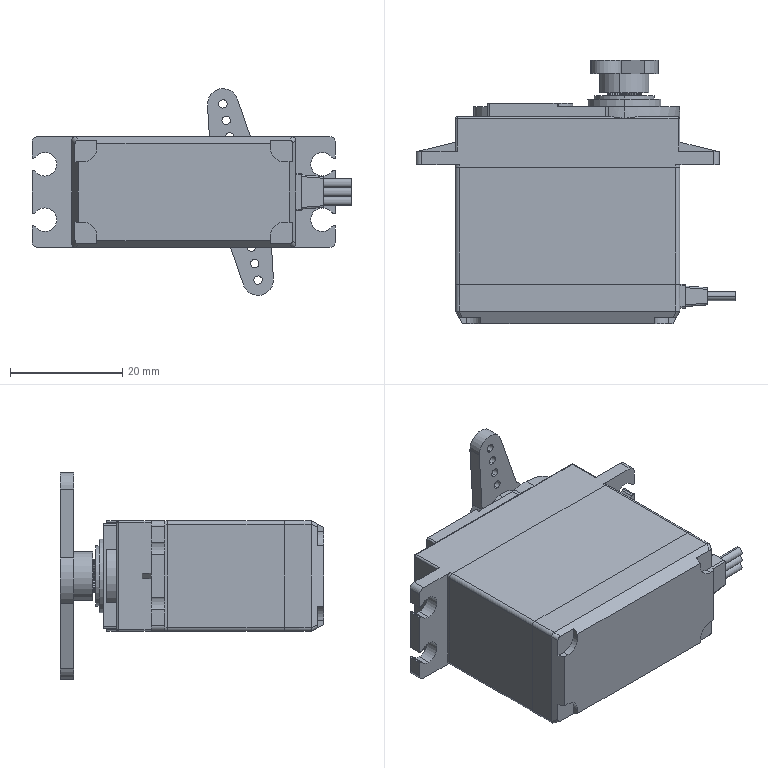Part | SolidWorks | 9 solids | 523 faces | box 56.95 x 46.85 x 36.783 mm | volume 5989 mm3 | plane 308 | cylinder 209 | spline 4 | cone 2 | commonest cylinder face diameters 0.6 x39 5.7 x36 5.95 x36 1.4 x16 1.5 x16 4.2 x12